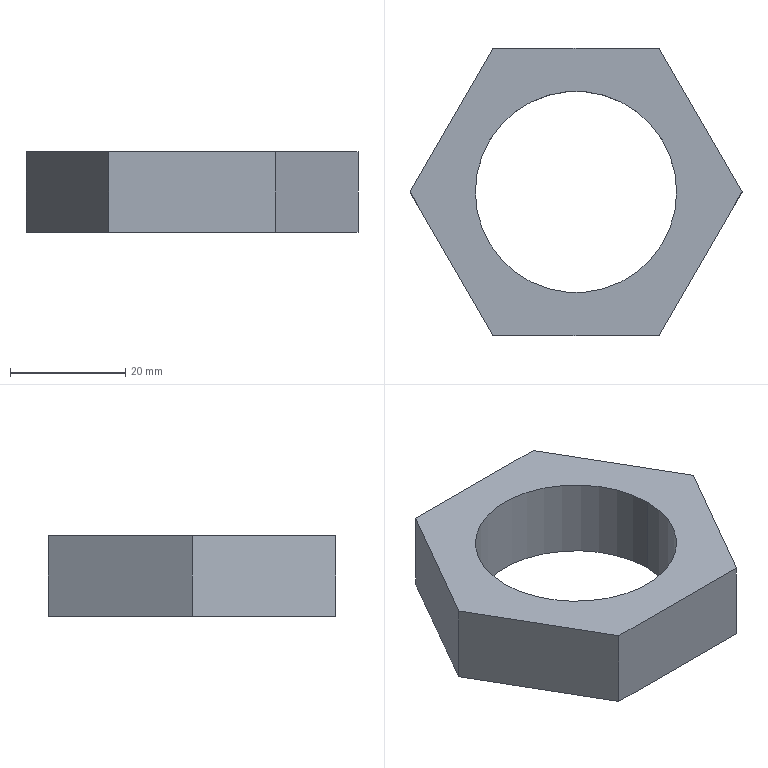Part | STEP file | TAN M35 BUOC 2 | 1 solid | 10 faces | box 57.735 x 50 x 14 mm | volume 16841 mm3 | plane 8 | cylinder 2 | commonest cylinder face diameters 35 x2
STEP:
#1=CARTESIAN_POINT('',(0.,0.,0.));
#2=DIRECTION('',(0.,0.,1.));
#3=DIRECTION('',(1.,0.,0.));
#4=AXIS2_PLACEMENT_3D('',#1,#2,#3);
#5=CARTESIAN_POINT('',(17.5,0.,0.));
#6=VERTEX_POINT('',#5);
#7=CARTESIAN_POINT('',(17.5,0.,14.));
#8=VERTEX_POINT('',#7);
#9=CARTESIAN_POINT('',(17.5,0.,0.));
#10=DIRECTION('',(0.,0.,1.));
#11=VECTOR('',#10,1.);
#12=LINE('',#9,#11);
#13=CARTESIAN_POINT('',(0.,0.,0.));
#14=DIRECTION('',(0.,0.,1.));
#15=DIRECTION('',(1.,0.,0.));
#16=AXIS2_PLACEMENT_3D('',#13,#14,#15);
#17=CYLINDRICAL_SURFACE('',#16,17.5);
#18=CARTESIAN_POINT('',(6.283,0.));
#19=DIRECTION('',(0.,1.));
#20=VECTOR('',#19,1.);
#21=LINE('',#18,#20);
#22=(GEOMETRIC_REPRESENTATION_CONTEXT(2)PARAMETRIC_REPRESENTATION_CONTEXT()REPRESENTATION_CONTEXT('',''));
#23=DEFINITIONAL_REPRESENTATION('',(#21),#22);
#24=PCURVE('',#17,#23);
#25=CARTESIAN_POINT('',(0.,0.,0.));
#26=DIRECTION('',(0.,0.,1.));
#27=DIRECTION('',(1.,0.,0.));
#28=AXIS2_PLACEMENT_3D('',#25,#26,#27);
#29=CYLINDRICAL_SURFACE('',#28,17.5);
#30=CARTESIAN_POINT('',(0.,0.));
#31=DIRECTION('',(0.,1.));
#32=VECTOR('',#31,1.);
#33=LINE('',#30,#32);
#34=(GEOMETRIC_REPRESENTATION_CONTEXT(2)PARAMETRIC_REPRESENTATION_CONTEXT()REPRESENTATION_CONTEXT('',''));
#35=DEFINITIONAL_REPRESENTATION('',(#33),#34);
#36=PCURVE('',#29,#35);
#37=SURFACE_CURVE('',#12,(#24,#36),.PCURVE_S1.);
#38=EDGE_CURVE('',#6,#8,#37,.T.);
#39=ORIENTED_EDGE('',*,*,#38,.T.);
#40=CARTESIAN_POINT('',(-17.5,0.,14.));
#41=VERTEX_POINT('',#40);
#42=CARTESIAN_POINT('',(0.,0.,14.));
#43=DIRECTION('',(0.,0.,-1.));
#44=DIRECTION('',(1.,0.,0.));
#45=AXIS2_PLACEMENT_3D('',#42,#43,#44);
#46=CIRCLE('',#45,17.5);
#47=CARTESIAN_POINT('',(6.283,14.));
#48=DIRECTION('',(-1.,0.));
#49=VECTOR('',#48,1.);
#50=LINE('',#47,#49);
#51=(GEOMETRIC_REPRESENTATION_CONTEXT(2)PARAMETRIC_REPRESENTATION_CONTEXT()REPRESENTATION_CONTEXT('',''));
#52=DEFINITIONAL_REPRESENTATION('',(#50),#51);
#53=PCURVE('',#17,#52);
#54=CARTESIAN_POINT('',(0.,0.,14.));
#55=DIRECTION('',(0.,0.,1.));
#56=DIRECTION('',(1.,0.,0.));
#57=AXIS2_PLACEMENT_3D('',#54,#55,#56);
#58=PLANE('',#57);
#59=CARTESIAN_POINT('',(17.5,0.));
#60=CARTESIAN_POINT('',(17.5,-30.311));
#61=CARTESIAN_POINT('',(-8.75,-15.155));
#62=CARTESIAN_POINT('',(-35.,0.));
#63=CARTESIAN_POINT('',(-8.75,15.155));
#64=CARTESIAN_POINT('',(17.5,30.311));
#65=CARTESIAN_POINT('',(17.5,0.));
#66=(BOUNDED_CURVE()B_SPLINE_CURVE(2,(#59,#60,#61,#62,#63,#64,#65),.UNSPECIFIED.,.T.,.F.)B_SPLINE_CURVE_WITH_KNOTS((1,2,2,2,2,1),(-2.094,0.,2.094,4.189,6.283,8.378),.UNSPECIFIED.)CURVE()GEOMETRIC_REPRESENTATION_ITEM()RATIONAL_B_SPLINE_CURVE((1.,0.5,1.,0.5,1.,0.5,1.))REPRESENTATION_ITEM(''));
#67=(GEOMETRIC_REPRESENTATION_CONTEXT(2)PARAMETRIC_REPRESENTATION_CONTEXT()REPRESENTATION_CONTEXT('',''));
#68=DEFINITIONAL_REPRESENTATION('',(#66),#67);
#69=PCURVE('',#58,#68);
#70=SURFACE_CURVE('',#46,(#53,#69),.PCURVE_S1.);
#71=EDGE_CURVE('',#8,#41,#70,.T.);
#72=ORIENTED_EDGE('',*,*,#71,.T.);
#73=CARTESIAN_POINT('',(-17.5,0.,0.));
#74=VERTEX_POINT('',#73);
#75=CARTESIAN_POINT('',(-17.5,0.,0.));
#76=DIRECTION('',(0.,0.,1.));
#77=VECTOR('',#76,1.);
#78=LINE('',#75,#77);
#79=CARTESIAN_POINT('',(3.142,0.));
#80=DIRECTION('',(0.,1.));
#81=VECTOR('',#80,1.);
#82=LINE('',#79,#81);
#83=(GEOMETRIC_REPRESENTATION_CONTEXT(2)PARAMETRIC_REPRESENTATION_CONTEXT()REPRESENTATION_CONTEXT('',''));
#84=DEFINITIONAL_REPRESENTATION('',(#82),#83);
#85=PCURVE('',#17,#84);
#86=CARTESIAN_POINT('',(3.142,0.));
#87=DIRECTION('',(0.,1.));
#88=VECTOR('',#87,1.);
#89=LINE('',#86,#88);
#90=(GEOMETRIC_REPRESENTATION_CONTEXT(2)PARAMETRIC_REPRESENTATION_CONTEXT()REPRESENTATION_CONTEXT('',''));
#91=DEFINITIONAL_REPRESENTATION('',(#89),#90);
#92=PCURVE('',#29,#91);
#93=SURFACE_CURVE('',#78,(#85,#92),.PCURVE_S1.);
#94=EDGE_CURVE('',#74,#41,#93,.T.);
#95=ORIENTED_EDGE('',*,*,#94,.F.);
#96=CARTESIAN_POINT('',(0.,0.,0.));
#97=DIRECTION('',(0.,0.,1.));
#98=DIRECTION('',(1.,0.,0.));
#99=AXIS2_PLACEMENT_3D('',#96,#97,#98);
#100=CIRCLE('',#99,17.5);
#101=CARTESIAN_POINT('',(0.,0.));
#102=DIRECTION('',(1.,0.));
#103=VECTOR('',#102,1.);
#104=LINE('',#101,#103);
#105=(GEOMETRIC_REPRESENTATION_CONTEXT(2)PARAMETRIC_REPRESENTATION_CONTEXT()REPRESENTATION_CONTEXT('',''));
#106=DEFINITIONAL_REPRESENTATION('',(#104),#105);
#107=PCURVE('',#17,#106);
#108=CARTESIAN_POINT('',(0.,0.,0.));
#109=DIRECTION('',(0.,0.,1.));
#110=DIRECTION('',(1.,0.,0.));
#111=AXIS2_PLACEMENT_3D('',#108,#109,#110);
#112=PLANE('',#111);
#113=CARTESIAN_POINT('',(0.,0.));
#114=DIRECTION('',(1.,0.));
#115=AXIS2_PLACEMENT_2D('',#113,#114);
#116=CIRCLE('',#115,17.5);
#117=(GEOMETRIC_REPRESENTATION_CONTEXT(2)PARAMETRIC_REPRESENTATION_CONTEXT()REPRESENTATION_CONTEXT('',''));
#118=DEFINITIONAL_REPRESENTATION('',(#116),#117);
#119=PCURVE('',#112,#118);
#120=SURFACE_CURVE('',#100,(#107,#119),.PCURVE_S1.);
#121=EDGE_CURVE('',#74,#6,#120,.T.);
#122=ORIENTED_EDGE('',*,*,#121,.T.);
#123=EDGE_LOOP('',(#39,#72,#95,#122));
#124=FACE_BOUND('',#123,.F.);
#125=ADVANCED_FACE('',(#124),#17,.F.);
#126=CARTESIAN_POINT('',(0.,0.,14.));
#127=DIRECTION('',(0.,0.,-1.));
#128=DIRECTION('',(1.,0.,0.));
#129=AXIS2_PLACEMENT_3D('',#126,#127,#128);
#130=CIRCLE('',#129,17.5);
#131=CARTESIAN_POINT('',(6.283,14.));
#132=DIRECTION('',(-1.,0.));
#133=VECTOR('',#132,1.);
#134=LINE('',#131,#133);
#135=(GEOMETRIC_REPRESENTATION_CONTEXT(2)PARAMETRIC_REPRESENTATION_CONTEXT()REPRESENTATION_CONTEXT('',''));
#136=DEFINITIONAL_REPRESENTATION('',(#134),#135);
#137=PCURVE('',#29,#136);
#138=CARTESIAN_POINT('',(17.5,0.));
#139=CARTESIAN_POINT('',(17.5,-30.311));
#140=CARTESIAN_POINT('',(-8.75,-15.155));
#141=CARTESIAN_POINT('',(-35.,0.));
#142=CARTESIAN_POINT('',(-8.75,15.155));
#143=CARTESIAN_POINT('',(17.5,30.311));
#144=CARTESIAN_POINT('',(17.5,0.));
#145=(BOUNDED_CURVE()B_SPLINE_CURVE(2,(#138,#139,#140,#141,#142,#143,#144),.UNSPECIFIED.,.T.,.F.)B_SPLINE_CURVE_WITH_KNOTS((1,2,2,2,2,1),(-2.094,0.,2.094,4.189,6.283,8.378),.UNSPECIFIED.)CURVE()GEOMETRIC_REPRESENTATION_ITEM()RATIONAL_B_SPLINE_CURVE((1.,0.5,1.,0.5,1.,0.5,1.))REPRESENTATION_ITEM(''));
#146=(GEOMETRIC_REPRESENTATION_CONTEXT(2)PARAMETRIC_REPRESENTATION_CONTEXT()REPRESENTATION_CONTEXT('',''));
#147=DEFINITIONAL_REPRESENTATION('',(#145),#146);
#148=PCURVE('',#58,#147);
#149=SURFACE_CURVE('',#130,(#137,#148),.PCURVE_S1.);
#150=EDGE_CURVE('',#41,#8,#149,.T.);
#151=ORIENTED_EDGE('',*,*,#150,.T.);
#152=ORIENTED_EDGE('',*,*,#38,.F.);
#153=CARTESIAN_POINT('',(0.,0.,0.));
#154=DIRECTION('',(0.,0.,1.));
#155=DIRECTION('',(1.,0.,0.));
#156=AXIS2_PLACEMENT_3D('',#153,#154,#155);
#157=CIRCLE('',#156,17.5);
#158=CARTESIAN_POINT('',(0.,0.));
#159=DIRECTION('',(1.,0.));
#160=VECTOR('',#159,1.);
#161=LINE('',#158,#160);
#162=(GEOMETRIC_REPRESENTATION_CONTEXT(2)PARAMETRIC_REPRESENTATION_CONTEXT()REPRESENTATION_CONTEXT('',''));
#163=DEFINITIONAL_REPRESENTATION('',(#161),#162);
#164=PCURVE('',#29,#163);
#165=CARTESIAN_POINT('',(0.,0.));
#166=DIRECTION('',(1.,0.));
#167=AXIS2_PLACEMENT_2D('',#165,#166);
#168=CIRCLE('',#167,17.5);
#169=(GEOMETRIC_REPRESENTATION_CONTEXT(2)PARAMETRIC_REPRESENTATION_CONTEXT()REPRESENTATION_CONTEXT('',''));
#170=DEFINITIONAL_REPRESENTATION('',(#168),#169);
#171=PCURVE('',#112,#170);
#172=SURFACE_CURVE('',#157,(#164,#171),.PCURVE_S1.);
#173=EDGE_CURVE('',#6,#74,#172,.T.);
#174=ORIENTED_EDGE('',*,*,#173,.T.);
#175=ORIENTED_EDGE('',*,*,#94,.T.);
#176=EDGE_LOOP('',(#151,#152,#174,#175));
#177=FACE_BOUND('',#176,.F.);
#178=ADVANCED_FACE('',(#177),#29,.F.);
#179=ORIENTED_EDGE('',*,*,#173,.T.);
#180=ORIENTED_EDGE('',*,*,#121,.T.);
#181=EDGE_LOOP('',(#179,#180));
#182=FACE_BOUND('',#181,.T.);
#183=CARTESIAN_POINT('',(14.434,25.,0.));
#184=VERTEX_POINT('',#183);
#185=CARTESIAN_POINT('',(-14.434,25.,0.));
#186=VERTEX_POINT('',#185);
#187=CARTESIAN_POINT('',(0.,25.,0.));
#188=DIRECTION('',(-1.,0.,0.));
#189=VECTOR('',#188,1.);
#190=LINE('',#187,#189);
#191=CARTESIAN_POINT('',(0.,25.));
#192=DIRECTION('',(-1.,0.));
#193=VECTOR('',#192,1.);
#194=LINE('',#191,#193);
#195=(GEOMETRIC_REPRESENTATION_CONTEXT(2)PARAMETRIC_REPRESENTATION_CONTEXT()REPRESENTATION_CONTEXT('',''));
#196=DEFINITIONAL_REPRESENTATION('',(#194),#195);
#197=PCURVE('',#112,#196);
#198=CARTESIAN_POINT('',(-14.434,25.,0.));
#199=DIRECTION('',(0.,1.,0.));
#200=DIRECTION('',(0.,0.,1.));
#201=AXIS2_PLACEMENT_3D('',#198,#199,#200);
#202=PLANE('',#201);
#203=CARTESIAN_POINT('',(0.,14.434));
#204=DIRECTION('',(0.,-1.));
#205=VECTOR('',#204,1.);
#206=LINE('',#203,#205);
#207=(GEOMETRIC_REPRESENTATION_CONTEXT(2)PARAMETRIC_REPRESENTATION_CONTEXT()REPRESENTATION_CONTEXT('',''));
#208=DEFINITIONAL_REPRESENTATION('',(#206),#207);
#209=PCURVE('',#202,#208);
#210=SURFACE_CURVE('',#190,(#197,#209),.PCURVE_S1.);
#211=EDGE_CURVE('',#184,#186,#210,.T.);
#212=ORIENTED_EDGE('',*,*,#211,.F.);
#213=CARTESIAN_POINT('',(28.868,0.,0.));
#214=VERTEX_POINT('',#213);
#215=CARTESIAN_POINT('',(28.868,0.,0.));
#216=DIRECTION('',(-0.5,0.866,0.));
#217=VECTOR('',#216,1.);
#218=LINE('',#215,#217);
#219=CARTESIAN_POINT('',(28.868,0.));
#220=DIRECTION('',(-0.5,0.866));
#221=VECTOR('',#220,1.);
#222=LINE('',#219,#221);
#223=(GEOMETRIC_REPRESENTATION_CONTEXT(2)PARAMETRIC_REPRESENTATION_CONTEXT()REPRESENTATION_CONTEXT('',''));
#224=DEFINITIONAL_REPRESENTATION('',(#222),#223);
#225=PCURVE('',#112,#224);
#226=CARTESIAN_POINT('',(14.434,25.,0.));
#227=DIRECTION('',(0.866,0.5,0.));
#228=DIRECTION('',(-0.5,0.866,0.));
#229=AXIS2_PLACEMENT_3D('',#226,#227,#228);
#230=PLANE('',#229);
#231=CARTESIAN_POINT('',(-28.868,0.));
#232=DIRECTION('',(1.,0.));
#233=VECTOR('',#232,1.);
#234=LINE('',#231,#233);
#235=(GEOMETRIC_REPRESENTATION_CONTEXT(2)PARAMETRIC_REPRESENTATION_CONTEXT()REPRESENTATION_CONTEXT('',''));
#236=DEFINITIONAL_REPRESENTATION('',(#234),#235);
#237=PCURVE('',#230,#236);
#238=SURFACE_CURVE('',#218,(#225,#237),.PCURVE_S1.);
#239=EDGE_CURVE('',#214,#184,#238,.T.);
#240=ORIENTED_EDGE('',*,*,#239,.F.);
#241=CARTESIAN_POINT('',(14.434,-25.,0.));
#242=VERTEX_POINT('',#241);
#243=CARTESIAN_POINT('',(14.434,-25.,0.));
#244=DIRECTION('',(0.5,0.866,0.));
#245=VECTOR('',#244,1.);
#246=LINE('',#243,#245);
#247=CARTESIAN_POINT('',(14.434,-25.));
#248=DIRECTION('',(0.5,0.866));
#249=VECTOR('',#248,1.);
#250=LINE('',#247,#249);
#251=(GEOMETRIC_REPRESENTATION_CONTEXT(2)PARAMETRIC_REPRESENTATION_CONTEXT()REPRESENTATION_CONTEXT('',''));
#252=DEFINITIONAL_REPRESENTATION('',(#250),#251);
#253=PCURVE('',#112,#252);
#254=CARTESIAN_POINT('',(28.868,0.,0.));
#255=DIRECTION('',(0.866,-0.5,0.));
#256=DIRECTION('',(0.5,0.866,0.));
#257=AXIS2_PLACEMENT_3D('',#254,#255,#256);
#258=PLANE('',#257);
#259=CARTESIAN_POINT('',(-28.868,0.));
#260=DIRECTION('',(1.,0.));
#261=VECTOR('',#260,1.);
#262=LINE('',#259,#261);
#263=(GEOMETRIC_REPRESENTATION_CONTEXT(2)PARAMETRIC_REPRESENTATION_CONTEXT()REPRESENTATION_CONTEXT('',''));
#264=DEFINITIONAL_REPRESENTATION('',(#262),#263);
#265=PCURVE('',#258,#264);
#266=SURFACE_CURVE('',#246,(#253,#265),.PCURVE_S1.);
#267=EDGE_CURVE('',#242,#214,#266,.T.);
#268=ORIENTED_EDGE('',*,*,#267,.F.);
#269=CARTESIAN_POINT('',(-14.434,-25.,0.));
#270=VERTEX_POINT('',#269);
#271=CARTESIAN_POINT('',(0.,-25.,0.));
#272=DIRECTION('',(1.,0.,0.));
#273=VECTOR('',#272,1.);
#274=LINE('',#271,#273);
#275=CARTESIAN_POINT('',(0.,-25.));
#276=DIRECTION('',(1.,0.));
#277=VECTOR('',#276,1.);
#278=LINE('',#275,#277);
#279=(GEOMETRIC_REPRESENTATION_CONTEXT(2)PARAMETRIC_REPRESENTATION_CONTEXT()REPRESENTATION_CONTEXT('',''));
#280=DEFINITIONAL_REPRESENTATION('',(#278),#279);
#281=PCURVE('',#112,#280);
#282=CARTESIAN_POINT('',(14.434,-25.,0.));
#283=DIRECTION('',(0.,-1.,0.));
#284=DIRECTION('',(0.,0.,-1.));
#285=AXIS2_PLACEMENT_3D('',#282,#283,#284);
#286=PLANE('',#285);
#287=CARTESIAN_POINT('',(0.,-14.434));
#288=DIRECTION('',(0.,1.));
#289=VECTOR('',#288,1.);
#290=LINE('',#287,#289);
#291=(GEOMETRIC_REPRESENTATION_CONTEXT(2)PARAMETRIC_REPRESENTATION_CONTEXT()REPRESENTATION_CONTEXT('',''));
#292=DEFINITIONAL_REPRESENTATION('',(#290),#291);
#293=PCURVE('',#286,#292);
#294=SURFACE_CURVE('',#274,(#281,#293),.PCURVE_S1.);
#295=EDGE_CURVE('',#270,#242,#294,.T.);
#296=ORIENTED_EDGE('',*,*,#295,.F.);
#297=CARTESIAN_POINT('',(-28.868,0.,0.));
#298=VERTEX_POINT('',#297);
#299=CARTESIAN_POINT('',(-28.868,0.,0.));
#300=DIRECTION('',(0.5,-0.866,0.));
#301=VECTOR('',#300,1.);
#302=LINE('',#299,#301);
#303=CARTESIAN_POINT('',(-28.868,0.));
#304=DIRECTION('',(0.5,-0.866));
#305=VECTOR('',#304,1.);
#306=LINE('',#303,#305);
#307=(GEOMETRIC_REPRESENTATION_CONTEXT(2)PARAMETRIC_REPRESENTATION_CONTEXT()REPRESENTATION_CONTEXT('',''));
#308=DEFINITIONAL_REPRESENTATION('',(#306),#307);
#309=PCURVE('',#112,#308);
#310=CARTESIAN_POINT('',(-14.434,-25.,0.));
#311=DIRECTION('',(-0.866,-0.5,0.));
#312=DIRECTION('',(0.5,-0.866,0.));
#313=AXIS2_PLACEMENT_3D('',#310,#311,#312);
#314=PLANE('',#313);
#315=CARTESIAN_POINT('',(-28.868,0.));
#316=DIRECTION('',(1.,0.));
#317=VECTOR('',#316,1.);
#318=LINE('',#315,#317);
#319=(GEOMETRIC_REPRESENTATION_CONTEXT(2)PARAMETRIC_REPRESENTATION_CONTEXT()REPRESENTATION_CONTEXT('',''));
#320=DEFINITIONAL_REPRESENTATION('',(#318),#319);
#321=PCURVE('',#314,#320);
#322=SURFACE_CURVE('',#302,(#309,#321),.PCURVE_S1.);
#323=EDGE_CURVE('',#298,#270,#322,.T.);
#324=ORIENTED_EDGE('',*,*,#323,.F.);
#325=CARTESIAN_POINT('',(-14.434,25.,0.));
#326=DIRECTION('',(-0.5,-0.866,0.));
#327=VECTOR('',#326,1.);
#328=LINE('',#325,#327);
#329=CARTESIAN_POINT('',(-14.434,25.));
#330=DIRECTION('',(-0.5,-0.866));
#331=VECTOR('',#330,1.);
#332=LINE('',#329,#331);
#333=(GEOMETRIC_REPRESENTATION_CONTEXT(2)PARAMETRIC_REPRESENTATION_CONTEXT()REPRESENTATION_CONTEXT('',''));
#334=DEFINITIONAL_REPRESENTATION('',(#332),#333);
#335=PCURVE('',#112,#334);
#336=CARTESIAN_POINT('',(-28.868,0.,0.));
#337=DIRECTION('',(-0.866,0.5,0.));
#338=DIRECTION('',(-0.5,-0.866,0.));
#339=AXIS2_PLACEMENT_3D('',#336,#337,#338);
#340=PLANE('',#339);
#341=CARTESIAN_POINT('',(-28.868,0.));
#342=DIRECTION('',(1.,0.));
#343=VECTOR('',#342,1.);
#344=LINE('',#341,#343);
#345=(GEOMETRIC_REPRESENTATION_CONTEXT(2)PARAMETRIC_REPRESENTATION_CONTEXT()REPRESENTATION_CONTEXT('',''));
#346=DEFINITIONAL_REPRESENTATION('',(#344),#345);
#347=PCURVE('',#340,#346);
#348=SURFACE_CURVE('',#328,(#335,#347),.PCURVE_S1.);
#349=EDGE_CURVE('',#186,#298,#348,.T.);
#350=ORIENTED_EDGE('',*,*,#349,.F.);
#351=EDGE_LOOP('',(#212,#240,#268,#296,#324,#350));
#352=FACE_BOUND('',#351,.T.);
#353=ADVANCED_FACE('',(#182,#352),#112,.F.);
#354=ORIENTED_EDGE('',*,*,#71,.T.);
#355=ORIENTED_EDGE('',*,*,#150,.T.);
#356=EDGE_LOOP('',(#354,#355));
#357=FACE_BOUND('',#356,.T.);
#358=CARTESIAN_POINT('',(14.434,-25.,14.));
#359=VERTEX_POINT('',#358);
#360=CARTESIAN_POINT('',(28.868,0.,14.));
#361=VERTEX_POINT('',#360);
#362=CARTESIAN_POINT('',(14.434,-25.,14.));
#363=DIRECTION('',(0.5,0.866,0.));
#364=VECTOR('',#363,1.);
#365=LINE('',#362,#364);
#366=CARTESIAN_POINT('',(14.434,-25.));
#367=DIRECTION('',(0.5,0.866));
#368=VECTOR('',#367,1.);
#369=LINE('',#366,#368);
#370=(GEOMETRIC_REPRESENTATION_CONTEXT(2)PARAMETRIC_REPRESENTATION_CONTEXT()REPRESENTATION_CONTEXT('',''));
#371=DEFINITIONAL_REPRESENTATION('',(#369),#370);
#372=PCURVE('',#58,#371);
#373=CARTESIAN_POINT('',(-28.868,14.));
#374=DIRECTION('',(1.,0.));
#375=VECTOR('',#374,1.);
#376=LINE('',#373,#375);
#377=(GEOMETRIC_REPRESENTATION_CONTEXT(2)PARAMETRIC_REPRESENTATION_CONTEXT()REPRESENTATION_CONTEXT('',''));
#378=DEFINITIONAL_REPRESENTATION('',(#376),#377);
#379=PCURVE('',#258,#378);
#380=SURFACE_CURVE('',#365,(#372,#379),.PCURVE_S1.);
#381=EDGE_CURVE('',#359,#361,#380,.T.);
#382=ORIENTED_EDGE('',*,*,#381,.T.);
#383=CARTESIAN_POINT('',(14.434,25.,14.));
#384=VERTEX_POINT('',#383);
#385=CARTESIAN_POINT('',(28.868,0.,14.));
#386=DIRECTION('',(-0.5,0.866,0.));
#387=VECTOR('',#386,1.);
#388=LINE('',#385,#387);
#389=CARTESIAN_POINT('',(28.868,0.));
#390=DIRECTION('',(-0.5,0.866));
#391=VECTOR('',#390,1.);
#392=LINE('',#389,#391);
#393=(GEOMETRIC_REPRESENTATION_CONTEXT(2)PARAMETRIC_REPRESENTATION_CONTEXT()REPRESENTATION_CONTEXT('',''));
#394=DEFINITIONAL_REPRESENTATION('',(#392),#393);
#395=PCURVE('',#58,#394);
#396=CARTESIAN_POINT('',(-28.868,14.));
#397=DIRECTION('',(1.,0.));
#398=VECTOR('',#397,1.);
#399=LINE('',#396,#398);
#400=(GEOMETRIC_REPRESENTATION_CONTEXT(2)PARAMETRIC_REPRESENTATION_CONTEXT()REPRESENTATION_CONTEXT('',''));
#401=DEFINITIONAL_REPRESENTATION('',(#399),#400);
#402=PCURVE('',#230,#401);
#403=SURFACE_CURVE('',#388,(#395,#402),.PCURVE_S1.);
#404=EDGE_CURVE('',#361,#384,#403,.T.);
#405=ORIENTED_EDGE('',*,*,#404,.T.);
#406=CARTESIAN_POINT('',(-14.434,25.,14.));
#407=VERTEX_POINT('',#406);
#408=CARTESIAN_POINT('',(0.,25.,14.));
#409=DIRECTION('',(-1.,0.,0.));
#410=VECTOR('',#409,1.);
#411=LINE('',#408,#410);
#412=CARTESIAN_POINT('',(0.,25.));
#413=DIRECTION('',(-1.,0.));
#414=VECTOR('',#413,1.);
#415=LINE('',#412,#414);
#416=(GEOMETRIC_REPRESENTATION_CONTEXT(2)PARAMETRIC_REPRESENTATION_CONTEXT()REPRESENTATION_CONTEXT('',''));
#417=DEFINITIONAL_REPRESENTATION('',(#415),#416);
#418=PCURVE('',#58,#417);
#419=CARTESIAN_POINT('',(14.,14.434));
#420=DIRECTION('',(0.,-1.));
#421=VECTOR('',#420,1.);
#422=LINE('',#419,#421);
#423=(GEOMETRIC_REPRESENTATION_CONTEXT(2)PARAMETRIC_REPRESENTATION_CONTEXT()REPRESENTATION_CONTEXT('',''));
#424=DEFINITIONAL_REPRESENTATION('',(#422),#423);
#425=PCURVE('',#202,#424);
#426=SURFACE_CURVE('',#411,(#418,#425),.PCURVE_S1.);
#427=EDGE_CURVE('',#384,#407,#426,.T.);
#428=ORIENTED_EDGE('',*,*,#427,.T.);
#429=CARTESIAN_POINT('',(-28.868,0.,14.));
#430=VERTEX_POINT('',#429);
#431=CARTESIAN_POINT('',(-14.434,25.,14.));
#432=DIRECTION('',(-0.5,-0.866,0.));
#433=VECTOR('',#432,1.);
#434=LINE('',#431,#433);
#435=CARTESIAN_POINT('',(-14.434,25.));
#436=DIRECTION('',(-0.5,-0.866));
#437=VECTOR('',#436,1.);
#438=LINE('',#435,#437);
#439=(GEOMETRIC_REPRESENTATION_CONTEXT(2)PARAMETRIC_REPRESENTATION_CONTEXT()REPRESENTATION_CONTEXT('',''));
#440=DEFINITIONAL_REPRESENTATION('',(#438),#439);
#441=PCURVE('',#58,#440);
#442=CARTESIAN_POINT('',(-28.868,14.));
#443=DIRECTION('',(1.,0.));
#444=VECTOR('',#443,1.);
#445=LINE('',#442,#444);
#446=(GEOMETRIC_REPRESENTATION_CONTEXT(2)PARAMETRIC_REPRESENTATION_CONTEXT()REPRESENTATION_CONTEXT('',''));
#447=DEFINITIONAL_REPRESENTATION('',(#445),#446);
#448=PCURVE('',#340,#447);
#449=SURFACE_CURVE('',#434,(#441,#448),.PCURVE_S1.);
#450=EDGE_CURVE('',#407,#430,#449,.T.);
#451=ORIENTED_EDGE('',*,*,#450,.T.);
#452=CARTESIAN_POINT('',(-14.434,-25.,14.));
#453=VERTEX_POINT('',#452);
#454=CARTESIAN_POINT('',(-28.868,0.,14.));
#455=DIRECTION('',(0.5,-0.866,0.));
#456=VECTOR('',#455,1.);
#457=LINE('',#454,#456);
#458=CARTESIAN_POINT('',(-28.868,0.));
#459=DIRECTION('',(0.5,-0.866));
#460=VECTOR('',#459,1.);
#461=LINE('',#458,#460);
#462=(GEOMETRIC_REPRESENTATION_CONTEXT(2)PARAMETRIC_REPRESENTATION_CONTEXT()REPRESENTATION_CONTEXT('',''));
#463=DEFINITIONAL_REPRESENTATION('',(#461),#462);
#464=PCURVE('',#58,#463);
#465=CARTESIAN_POINT('',(-28.868,14.));
#466=DIRECTION('',(1.,0.));
#467=VECTOR('',#466,1.);
#468=LINE('',#465,#467);
#469=(GEOMETRIC_REPRESENTATION_CONTEXT(2)PARAMETRIC_REPRESENTATION_CONTEXT()REPRESENTATION_CONTEXT('',''));
#470=DEFINITIONAL_REPRESENTATION('',(#468),#469);
#471=PCURVE('',#314,#470);
#472=SURFACE_CURVE('',#457,(#464,#471),.PCURVE_S1.);
#473=EDGE_CURVE('',#430,#453,#472,.T.);
#474=ORIENTED_EDGE('',*,*,#473,.T.);
#475=CARTESIAN_POINT('',(0.,-25.,14.));
#476=DIRECTION('',(1.,0.,0.));
#477=VECTOR('',#476,1.);
#478=LINE('',#475,#477);
#479=CARTESIAN_POINT('',(0.,-25.));
#480=DIRECTION('',(1.,0.));
#481=VECTOR('',#480,1.);
#482=LINE('',#479,#481);
#483=(GEOMETRIC_REPRESENTATION_CONTEXT(2)PARAMETRIC_REPRESENTATION_CONTEXT()REPRESENTATION_CONTEXT('',''));
#484=DEFINITIONAL_REPRESENTATION('',(#482),#483);
#485=PCURVE('',#58,#484);
#486=CARTESIAN_POINT('',(-14.,-14.434));
#487=DIRECTION('',(0.,1.));
#488=VECTOR('',#487,1.);
#489=LINE('',#486,#488);
#490=(GEOMETRIC_REPRESENTATION_CONTEXT(2)PARAMETRIC_REPRESENTATION_CONTEXT()REPRESENTATION_CONTEXT('',''));
#491=DEFINITIONAL_REPRESENTATION('',(#489),#490);
#492=PCURVE('',#286,#491);
#493=SURFACE_CURVE('',#478,(#485,#492),.PCURVE_S1.);
#494=EDGE_CURVE('',#453,#359,#493,.T.);
#495=ORIENTED_EDGE('',*,*,#494,.T.);
#496=EDGE_LOOP('',(#382,#405,#428,#451,#474,#495));
#497=FACE_BOUND('',#496,.T.);
#498=ADVANCED_FACE('',(#357,#497),#58,.T.);
#499=ORIENTED_EDGE('',*,*,#349,.T.);
#500=CARTESIAN_POINT('',(-28.868,0.,0.));
#501=DIRECTION('',(0.,0.,1.));
#502=VECTOR('',#501,1.);
#503=LINE('',#500,#502);
#504=CARTESIAN_POINT('',(0.,0.));
#505=DIRECTION('',(0.,1.));
#506=VECTOR('',#505,1.);
#507=LINE('',#504,#506);
#508=(GEOMETRIC_REPRESENTATION_CONTEXT(2)PARAMETRIC_REPRESENTATION_CONTEXT()REPRESENTATION_CONTEXT('',''));
#509=DEFINITIONAL_REPRESENTATION('',(#507),#508);
#510=PCURVE('',#340,#509);
#511=CARTESIAN_POINT('',(-28.868,0.));
#512=DIRECTION('',(0.,1.));
#513=VECTOR('',#512,1.);
#514=LINE('',#511,#513);
#515=(GEOMETRIC_REPRESENTATION_CONTEXT(2)PARAMETRIC_REPRESENTATION_CONTEXT()REPRESENTATION_CONTEXT('',''));
#516=DEFINITIONAL_REPRESENTATION('',(#514),#515);
#517=PCURVE('',#314,#516);
#518=SURFACE_CURVE('',#503,(#510,#517),.PCURVE_S1.);
#519=EDGE_CURVE('',#298,#430,#518,.T.);
#520=ORIENTED_EDGE('',*,*,#519,.T.);
#521=ORIENTED_EDGE('',*,*,#450,.F.);
#522=CARTESIAN_POINT('',(-14.434,25.,0.));
#523=DIRECTION('',(0.,0.,-1.));
#524=VECTOR('',#523,1.);
#525=LINE('',#522,#524);
#526=CARTESIAN_POINT('',(-28.868,0.));
#527=DIRECTION('',(0.,-1.));
#528=VECTOR('',#527,1.);
#529=LINE('',#526,#528);
#530=(GEOMETRIC_REPRESENTATION_CONTEXT(2)PARAMETRIC_REPRESENTATION_CONTEXT()REPRESENTATION_CONTEXT('',''));
#531=DEFINITIONAL_REPRESENTATION('',(#529),#530);
#532=PCURVE('',#340,#531);
#533=CARTESIAN_POINT('',(0.,0.));
#534=DIRECTION('',(-1.,0.));
#535=VECTOR('',#534,1.);
#536=LINE('',#533,#535);
#537=(GEOMETRIC_REPRESENTATION_CONTEXT(2)PARAMETRIC_REPRESENTATION_CONTEXT()REPRESENTATION_CONTEXT('',''));
#538=DEFINITIONAL_REPRESENTATION('',(#536),#537);
#539=PCURVE('',#202,#538);
#540=SURFACE_CURVE('',#525,(#532,#539),.PCURVE_S1.);
#541=EDGE_CURVE('',#407,#186,#540,.T.);
#542=ORIENTED_EDGE('',*,*,#541,.T.);
#543=EDGE_LOOP('',(#499,#520,#521,#542));
#544=FACE_BOUND('',#543,.T.);
#545=ADVANCED_FACE('',(#544),#340,.T.);
#546=ORIENTED_EDGE('',*,*,#211,.T.);
#547=ORIENTED_EDGE('',*,*,#541,.F.);
#548=ORIENTED_EDGE('',*,*,#427,.F.);
#549=CARTESIAN_POINT('',(14.434,25.,0.));
#550=DIRECTION('',(0.,0.,-1.));
#551=VECTOR('',#550,1.);
#552=LINE('',#549,#551);
#553=CARTESIAN_POINT('',(0.,28.868));
#554=DIRECTION('',(-1.,0.));
#555=VECTOR('',#554,1.);
#556=LINE('',#553,#555);
#557=(GEOMETRIC_REPRESENTATION_CONTEXT(2)PARAMETRIC_REPRESENTATION_CONTEXT()REPRESENTATION_CONTEXT('',''));
#558=DEFINITIONAL_REPRESENTATION('',(#556),#557);
#559=PCURVE('',#202,#558);
#560=CARTESIAN_POINT('',(0.,0.));
#561=DIRECTION('',(0.,-1.));
#562=VECTOR('',#561,1.);
#563=LINE('',#560,#562);
#564=(GEOMETRIC_REPRESENTATION_CONTEXT(2)PARAMETRIC_REPRESENTATION_CONTEXT()REPRESENTATION_CONTEXT('',''));
#565=DEFINITIONAL_REPRESENTATION('',(#563),#564);
#566=PCURVE('',#230,#565);
#567=SURFACE_CURVE('',#552,(#559,#566),.PCURVE_S1.);
#568=EDGE_CURVE('',#384,#184,#567,.T.);
#569=ORIENTED_EDGE('',*,*,#568,.T.);
#570=EDGE_LOOP('',(#546,#547,#548,#569));
#571=FACE_BOUND('',#570,.T.);
#572=ADVANCED_FACE('',(#571),#202,.T.);
#573=ORIENTED_EDGE('',*,*,#239,.T.);
#574=ORIENTED_EDGE('',*,*,#568,.F.);
#575=ORIENTED_EDGE('',*,*,#404,.F.);
#576=CARTESIAN_POINT('',(28.868,0.,0.));
#577=DIRECTION('',(0.,0.,-1.));
#578=VECTOR('',#577,1.);
#579=LINE('',#576,#578);
#580=CARTESIAN_POINT('',(-28.868,0.));
#581=DIRECTION('',(0.,-1.));
#582=VECTOR('',#581,1.);
#583=LINE('',#580,#582);
#584=(GEOMETRIC_REPRESENTATION_CONTEXT(2)PARAMETRIC_REPRESENTATION_CONTEXT()REPRESENTATION_CONTEXT('',''));
#585=DEFINITIONAL_REPRESENTATION('',(#583),#584);
#586=PCURVE('',#230,#585);
#587=CARTESIAN_POINT('',(0.,0.));
#588=DIRECTION('',(0.,-1.));
#589=VECTOR('',#588,1.);
#590=LINE('',#587,#589);
#591=(GEOMETRIC_REPRESENTATION_CONTEXT(2)PARAMETRIC_REPRESENTATION_CONTEXT()REPRESENTATION_CONTEXT('',''));
#592=DEFINITIONAL_REPRESENTATION('',(#590),#591);
#593=PCURVE('',#258,#592);
#594=SURFACE_CURVE('',#579,(#586,#593),.PCURVE_S1.);
#595=EDGE_CURVE('',#361,#214,#594,.T.);
#596=ORIENTED_EDGE('',*,*,#595,.T.);
#597=EDGE_LOOP('',(#573,#574,#575,#596));
#598=FACE_BOUND('',#597,.T.);
#599=ADVANCED_FACE('',(#598),#230,.T.);
#600=ORIENTED_EDGE('',*,*,#267,.T.);
#601=ORIENTED_EDGE('',*,*,#595,.F.);
#602=ORIENTED_EDGE('',*,*,#381,.F.);
#603=CARTESIAN_POINT('',(14.434,-25.,0.));
#604=DIRECTION('',(0.,0.,-1.));
#605=VECTOR('',#604,1.);
#606=LINE('',#603,#605);
#607=CARTESIAN_POINT('',(-28.868,0.));
#608=DIRECTION('',(0.,-1.));
#609=VECTOR('',#608,1.);
#610=LINE('',#607,#609);
#611=(GEOMETRIC_REPRESENTATION_CONTEXT(2)PARAMETRIC_REPRESENTATION_CONTEXT()REPRESENTATION_CONTEXT('',''));
#612=DEFINITIONAL_REPRESENTATION('',(#610),#611);
#613=PCURVE('',#258,#612);
#614=CARTESIAN_POINT('',(0.,0.));
#615=DIRECTION('',(1.,0.));
#616=VECTOR('',#615,1.);
#617=LINE('',#614,#616);
#618=(GEOMETRIC_REPRESENTATION_CONTEXT(2)PARAMETRIC_REPRESENTATION_CONTEXT()REPRESENTATION_CONTEXT('',''));
#619=DEFINITIONAL_REPRESENTATION('',(#617),#618);
#620=PCURVE('',#286,#619);
#621=SURFACE_CURVE('',#606,(#613,#620),.PCURVE_S1.);
#622=EDGE_CURVE('',#359,#242,#621,.T.);
#623=ORIENTED_EDGE('',*,*,#622,.T.);
#624=EDGE_LOOP('',(#600,#601,#602,#623));
#625=FACE_BOUND('',#624,.T.);
#626=ADVANCED_FACE('',(#625),#258,.T.);
#627=ORIENTED_EDGE('',*,*,#295,.T.);
#628=ORIENTED_EDGE('',*,*,#622,.F.);
#629=ORIENTED_EDGE('',*,*,#494,.F.);
#630=CARTESIAN_POINT('',(-14.434,-25.,0.));
#631=DIRECTION('',(0.,0.,-1.));
#632=VECTOR('',#631,1.);
#633=LINE('',#630,#632);
#634=CARTESIAN_POINT('',(0.,-28.868));
#635=DIRECTION('',(1.,0.));
#636=VECTOR('',#635,1.);
#637=LINE('',#634,#636);
#638=(GEOMETRIC_REPRESENTATION_CONTEXT(2)PARAMETRIC_REPRESENTATION_CONTEXT()REPRESENTATION_CONTEXT('',''));
#639=DEFINITIONAL_REPRESENTATION('',(#637),#638);
#640=PCURVE('',#286,#639);
#641=CARTESIAN_POINT('',(0.,0.));
#642=DIRECTION('',(0.,-1.));
#643=VECTOR('',#642,1.);
#644=LINE('',#641,#643);
#645=(GEOMETRIC_REPRESENTATION_CONTEXT(2)PARAMETRIC_REPRESENTATION_CONTEXT()REPRESENTATION_CONTEXT('',''));
#646=DEFINITIONAL_REPRESENTATION('',(#644),#645);
#647=PCURVE('',#314,#646);
#648=SURFACE_CURVE('',#633,(#640,#647),.PCURVE_S1.);
#649=EDGE_CURVE('',#453,#270,#648,.T.);
#650=ORIENTED_EDGE('',*,*,#649,.T.);
#651=EDGE_LOOP('',(#627,#628,#629,#650));
#652=FACE_BOUND('',#651,.T.);
#653=ADVANCED_FACE('',(#652),#286,.T.);
#654=ORIENTED_EDGE('',*,*,#323,.T.);
#655=ORIENTED_EDGE('',*,*,#649,.F.);
#656=ORIENTED_EDGE('',*,*,#473,.F.);
#657=ORIENTED_EDGE('',*,*,#519,.F.);
#658=EDGE_LOOP('',(#654,#655,#656,#657));
#659=FACE_BOUND('',#658,.T.);
#660=ADVANCED_FACE('',(#659),#314,.T.);
#661=CLOSED_SHELL('',(#125,#178,#353,#498,#545,#572,#599,#626,#653,#660));
#662=MANIFOLD_SOLID_BREP('',#661);
#663=(LENGTH_UNIT()NAMED_UNIT(*)SI_UNIT(.MILLI.,.METRE.));
#664=UNCERTAINTY_MEASURE_WITH_UNIT(LENGTH_MEASURE(0.0000001),#663,'','');
#665=(NAMED_UNIT(*)PLANE_ANGLE_UNIT()SI_UNIT($,.RADIAN.));
#666=(NAMED_UNIT(*)SI_UNIT($,.STERADIAN.)SOLID_ANGLE_UNIT());
#667=(GEOMETRIC_REPRESENTATION_CONTEXT(3)GLOBAL_UNCERTAINTY_ASSIGNED_CONTEXT((#664))GLOBAL_UNIT_ASSIGNED_CONTEXT((#663,#665,#666))REPRESENTATION_CONTEXT('',''));
#668=ADVANCED_BREP_SHAPE_REPRESENTATION('',(#4,#662),#667);